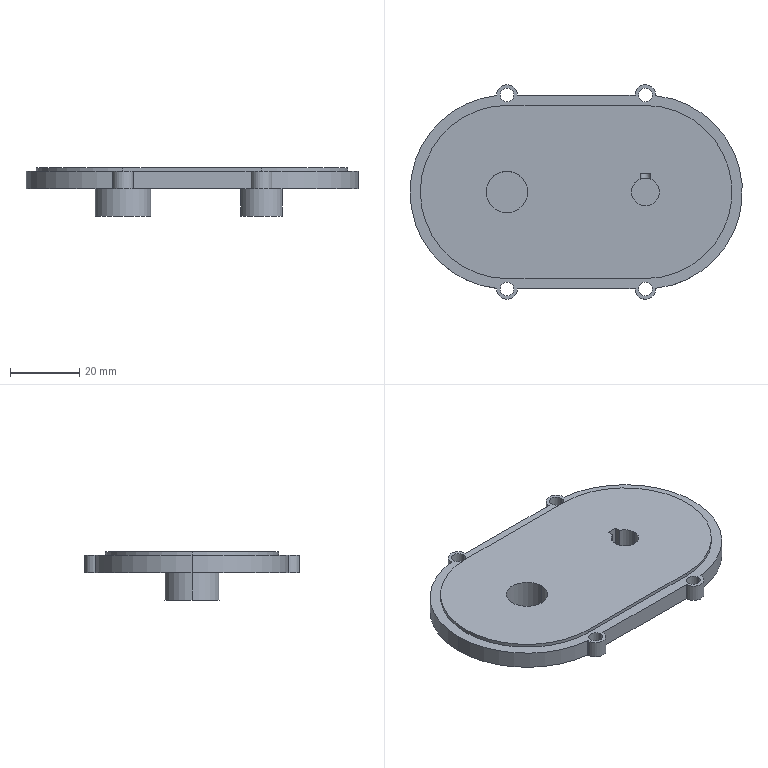Part | SolidWorks | features ICE 6, Extrusion 1 | 1 solid | 43 faces | box 96 x 62 x 14 mm | volume 28190 mm3 | cylinder 29 | plane 14 | commonest cylinder face diameters 4 x8 6 x6 12 x4 50 x3 56 x3 8 x2
STEP:
#1=CARTESIAN_POINT('',(-26.,0.,-5.));
#2=VERTEX_POINT('',#1);
#3=CARTESIAN_POINT('',(-14.,0.,-5.));
#4=VERTEX_POINT('',#3);
#5=CARTESIAN_POINT('',(-20.,0.,-5.));
#6=DIRECTION('',(0.,0.,1.));
#7=DIRECTION('',(1.,0.,0.));
#8=AXIS2_PLACEMENT_3D('',#5,#6,#7);
#9=CIRCLE('',#8,6.);
#10=EDGE_CURVE('',#2,#4,#9,.T.);
#11=ORIENTED_EDGE('',*,*,#10,.F.);
#12=CARTESIAN_POINT('',(-26.,0.,6.));
#13=VERTEX_POINT('',#12);
#14=CARTESIAN_POINT('',(-26.,0.,-5.));
#15=DIRECTION('',(0.,0.,1.));
#16=VECTOR('',#15,1000.);
#17=LINE('',#14,#16);
#18=EDGE_CURVE('',#2,#13,#17,.T.);
#19=ORIENTED_EDGE('',*,*,#18,.T.);
#20=CARTESIAN_POINT('',(-14.,0.,6.));
#21=VERTEX_POINT('',#20);
#22=CARTESIAN_POINT('',(-20.,0.,6.));
#23=DIRECTION('',(0.,0.,1.));
#24=DIRECTION('',(1.,0.,0.));
#25=AXIS2_PLACEMENT_3D('',#22,#23,#24);
#26=CIRCLE('',#25,6.);
#27=EDGE_CURVE('',#13,#21,#26,.T.);
#28=ORIENTED_EDGE('',*,*,#27,.T.);
#29=CARTESIAN_POINT('',(-14.,0.,-5.));
#30=DIRECTION('',(0.,0.,1.));
#31=VECTOR('',#30,1000.);
#32=LINE('',#29,#31);
#33=EDGE_CURVE('',#4,#21,#32,.T.);
#34=ORIENTED_EDGE('',*,*,#33,.F.);
#35=EDGE_LOOP('',(#11,#19,#28,#34));
#36=FACE_OUTER_BOUND('',#35,.T.);
#37=CARTESIAN_POINT('',(-20.,0.,-5.));
#38=DIRECTION('',(0.,0.,1.));
#39=DIRECTION('',(1.,0.,0.));
#40=AXIS2_PLACEMENT_3D('',#37,#38,#39);
#41=CYLINDRICAL_SURFACE('',#40,6.);
#42=ADVANCED_FACE('',(#36),#41,.F.);
#43=CARTESIAN_POINT('',(16.,0.,-5.));
#44=VERTEX_POINT('',#43);
#45=CARTESIAN_POINT('',(24.,0.,-5.));
#46=VERTEX_POINT('',#45);
#47=CARTESIAN_POINT('',(20.,0.,-5.));
#48=DIRECTION('',(0.,0.,1.));
#49=DIRECTION('',(1.,0.,0.));
#50=AXIS2_PLACEMENT_3D('',#47,#48,#49);
#51=CIRCLE('',#50,4.);
#52=EDGE_CURVE('',#44,#46,#51,.T.);
#53=ORIENTED_EDGE('',*,*,#52,.F.);
#54=CARTESIAN_POINT('',(16.,0.,6.));
#55=VERTEX_POINT('',#54);
#56=CARTESIAN_POINT('',(16.,0.,-5.));
#57=DIRECTION('',(0.,0.,1.));
#58=VECTOR('',#57,1000.);
#59=LINE('',#56,#58);
#60=EDGE_CURVE('',#44,#55,#59,.T.);
#61=ORIENTED_EDGE('',*,*,#60,.T.);
#62=CARTESIAN_POINT('',(24.,0.,6.));
#63=VERTEX_POINT('',#62);
#64=CARTESIAN_POINT('',(20.,0.,6.));
#65=DIRECTION('',(0.,0.,1.));
#66=DIRECTION('',(1.,0.,0.));
#67=AXIS2_PLACEMENT_3D('',#64,#65,#66);
#68=CIRCLE('',#67,4.);
#69=EDGE_CURVE('',#55,#63,#68,.T.);
#70=ORIENTED_EDGE('',*,*,#69,.T.);
#71=CARTESIAN_POINT('',(24.,0.,-5.));
#72=DIRECTION('',(0.,0.,1.));
#73=VECTOR('',#72,1000.);
#74=LINE('',#71,#73);
#75=EDGE_CURVE('',#46,#63,#74,.T.);
#76=ORIENTED_EDGE('',*,*,#75,.F.);
#77=EDGE_LOOP('',(#53,#61,#70,#76));
#78=FACE_OUTER_BOUND('',#77,.T.);
#79=CARTESIAN_POINT('',(20.,0.,-5.));
#80=DIRECTION('',(0.,0.,1.));
#81=DIRECTION('',(1.,0.,0.));
#82=AXIS2_PLACEMENT_3D('',#79,#80,#81);
#83=CYLINDRICAL_SURFACE('',#82,4.);
#84=ADVANCED_FACE('',(#78),#83,.F.);
#85=CARTESIAN_POINT('',(-28.,0.,-8.));
#86=VERTEX_POINT('',#85);
#87=CARTESIAN_POINT('',(-12.,0.,-8.));
#88=VERTEX_POINT('',#87);
#89=CARTESIAN_POINT('',(-20.,0.,-8.));
#90=DIRECTION('',(0.,0.,-1.));
#91=DIRECTION('',(-1.,0.,0.));
#92=AXIS2_PLACEMENT_3D('',#89,#90,#91);
#93=CIRCLE('',#92,8.);
#94=EDGE_CURVE('',#86,#88,#93,.T.);
#95=ORIENTED_EDGE('',*,*,#94,.F.);
#96=CARTESIAN_POINT('',(-28.,0.,0.));
#97=VERTEX_POINT('',#96);
#98=CARTESIAN_POINT('',(-28.,0.,-8.));
#99=DIRECTION('',(0.,0.,1.));
#100=VECTOR('',#99,1000.);
#101=LINE('',#98,#100);
#102=EDGE_CURVE('',#86,#97,#101,.T.);
#103=ORIENTED_EDGE('',*,*,#102,.T.);
#104=CARTESIAN_POINT('',(-12.,0.,0.));
#105=VERTEX_POINT('',#104);
#106=CARTESIAN_POINT('',(-20.,0.,0.));
#107=DIRECTION('',(0.,0.,-1.));
#108=DIRECTION('',(1.,0.,0.));
#109=AXIS2_PLACEMENT_3D('',#106,#107,#108);
#110=CIRCLE('',#109,8.);
#111=EDGE_CURVE('',#97,#105,#110,.T.);
#112=ORIENTED_EDGE('',*,*,#111,.T.);
#113=CARTESIAN_POINT('',(-12.,0.,-8.));
#114=DIRECTION('',(0.,0.,1.));
#115=VECTOR('',#114,1000.);
#116=LINE('',#113,#115);
#117=EDGE_CURVE('',#88,#105,#116,.T.);
#118=ORIENTED_EDGE('',*,*,#117,.F.);
#119=EDGE_LOOP('',(#95,#103,#112,#118));
#120=FACE_OUTER_BOUND('',#119,.T.);
#121=CARTESIAN_POINT('',(-20.,0.,-8.));
#122=DIRECTION('',(0.,0.,1.));
#123=DIRECTION('',(1.,0.,0.));
#124=AXIS2_PLACEMENT_3D('',#121,#122,#123);
#125=CYLINDRICAL_SURFACE('',#124,8.);
#126=ADVANCED_FACE('',(#120),#125,.T.);
#127=CARTESIAN_POINT('',(14.,0.,-8.));
#128=VERTEX_POINT('',#127);
#129=CARTESIAN_POINT('',(26.,0.,-8.));
#130=VERTEX_POINT('',#129);
#131=CARTESIAN_POINT('',(20.,0.,-8.));
#132=DIRECTION('',(0.,0.,-1.));
#133=DIRECTION('',(-1.,0.,0.));
#134=AXIS2_PLACEMENT_3D('',#131,#132,#133);
#135=CIRCLE('',#134,6.);
#136=EDGE_CURVE('',#128,#130,#135,.T.);
#137=ORIENTED_EDGE('',*,*,#136,.F.);
#138=CARTESIAN_POINT('',(14.,0.,0.));
#139=VERTEX_POINT('',#138);
#140=CARTESIAN_POINT('',(14.,0.,-8.));
#141=DIRECTION('',(0.,0.,1.));
#142=VECTOR('',#141,1000.);
#143=LINE('',#140,#142);
#144=EDGE_CURVE('',#128,#139,#143,.T.);
#145=ORIENTED_EDGE('',*,*,#144,.T.);
#146=CARTESIAN_POINT('',(26.,0.,0.));
#147=VERTEX_POINT('',#146);
#148=CARTESIAN_POINT('',(20.,0.,0.));
#149=DIRECTION('',(0.,0.,-1.));
#150=DIRECTION('',(1.,0.,0.));
#151=AXIS2_PLACEMENT_3D('',#148,#149,#150);
#152=CIRCLE('',#151,6.);
#153=EDGE_CURVE('',#139,#147,#152,.T.);
#154=ORIENTED_EDGE('',*,*,#153,.T.);
#155=CARTESIAN_POINT('',(26.,0.,-8.));
#156=DIRECTION('',(0.,0.,1.));
#157=VECTOR('',#156,1000.);
#158=LINE('',#155,#157);
#159=EDGE_CURVE('',#130,#147,#158,.T.);
#160=ORIENTED_EDGE('',*,*,#159,.F.);
#161=EDGE_LOOP('',(#137,#145,#154,#160));
#162=FACE_OUTER_BOUND('',#161,.T.);
#163=CARTESIAN_POINT('',(20.,0.,-8.));
#164=DIRECTION('',(0.,0.,1.));
#165=DIRECTION('',(1.,0.,0.));
#166=AXIS2_PLACEMENT_3D('',#163,#164,#165);
#167=CYLINDRICAL_SURFACE('',#166,6.);
#168=ADVANCED_FACE('',(#162),#167,.T.);
#169=CARTESIAN_POINT('',(-18.,28.,5.));
#170=VERTEX_POINT('',#169);
#171=CARTESIAN_POINT('',(-22.,28.,5.));
#172=VERTEX_POINT('',#171);
#173=CARTESIAN_POINT('',(-20.,28.,5.));
#174=DIRECTION('',(0.,0.,-1.));
#175=DIRECTION('',(-1.,0.,0.));
#176=AXIS2_PLACEMENT_3D('',#173,#174,#175);
#177=CIRCLE('',#176,2.);
#178=EDGE_CURVE('',#170,#172,#177,.T.);
#179=ORIENTED_EDGE('',*,*,#178,.F.);
#180=CARTESIAN_POINT('',(-18.,28.,0.));
#181=VERTEX_POINT('',#180);
#182=CARTESIAN_POINT('',(-18.,28.,5.));
#183=DIRECTION('',(0.,0.,-1.));
#184=VECTOR('',#183,1000.);
#185=LINE('',#182,#184);
#186=EDGE_CURVE('',#170,#181,#185,.T.);
#187=ORIENTED_EDGE('',*,*,#186,.T.);
#188=CARTESIAN_POINT('',(-22.,28.,0.));
#189=VERTEX_POINT('',#188);
#190=CARTESIAN_POINT('',(-20.,28.,0.));
#191=DIRECTION('',(0.,0.,-1.));
#192=DIRECTION('',(-1.,0.,0.));
#193=AXIS2_PLACEMENT_3D('',#190,#191,#192);
#194=CIRCLE('',#193,2.);
#195=EDGE_CURVE('',#181,#189,#194,.T.);
#196=ORIENTED_EDGE('',*,*,#195,.T.);
#197=CARTESIAN_POINT('',(-22.,28.,5.));
#198=DIRECTION('',(0.,0.,-1.));
#199=VECTOR('',#198,1000.);
#200=LINE('',#197,#199);
#201=EDGE_CURVE('',#172,#189,#200,.T.);
#202=ORIENTED_EDGE('',*,*,#201,.F.);
#203=EDGE_LOOP('',(#179,#187,#196,#202));
#204=FACE_OUTER_BOUND('',#203,.T.);
#205=CARTESIAN_POINT('',(-20.,28.,5.));
#206=DIRECTION('',(0.,0.,-1.));
#207=DIRECTION('',(-1.,0.,0.));
#208=AXIS2_PLACEMENT_3D('',#205,#206,#207);
#209=CYLINDRICAL_SURFACE('',#208,2.);
#210=ADVANCED_FACE('',(#204),#209,.F.);
#211=CARTESIAN_POINT('',(22.,-28.,5.));
#212=VERTEX_POINT('',#211);
#213=CARTESIAN_POINT('',(18.,-28.,5.));
#214=VERTEX_POINT('',#213);
#215=CARTESIAN_POINT('',(20.,-28.,5.));
#216=DIRECTION('',(0.,0.,-1.));
#217=DIRECTION('',(-1.,0.,0.));
#218=AXIS2_PLACEMENT_3D('',#215,#216,#217);
#219=CIRCLE('',#218,2.);
#220=EDGE_CURVE('',#212,#214,#219,.T.);
#221=ORIENTED_EDGE('',*,*,#220,.F.);
#222=CARTESIAN_POINT('',(22.,-28.,0.));
#223=VERTEX_POINT('',#222);
#224=CARTESIAN_POINT('',(22.,-28.,5.));
#225=DIRECTION('',(0.,0.,-1.));
#226=VECTOR('',#225,1000.);
#227=LINE('',#224,#226);
#228=EDGE_CURVE('',#212,#223,#227,.T.);
#229=ORIENTED_EDGE('',*,*,#228,.T.);
#230=CARTESIAN_POINT('',(18.,-28.,0.));
#231=VERTEX_POINT('',#230);
#232=CARTESIAN_POINT('',(20.,-28.,0.));
#233=DIRECTION('',(0.,0.,-1.));
#234=DIRECTION('',(-1.,0.,0.));
#235=AXIS2_PLACEMENT_3D('',#232,#233,#234);
#236=CIRCLE('',#235,2.);
#237=EDGE_CURVE('',#223,#231,#236,.T.);
#238=ORIENTED_EDGE('',*,*,#237,.T.);
#239=CARTESIAN_POINT('',(18.,-28.,5.));
#240=DIRECTION('',(0.,0.,-1.));
#241=VECTOR('',#240,1000.);
#242=LINE('',#239,#241);
#243=EDGE_CURVE('',#214,#231,#242,.T.);
#244=ORIENTED_EDGE('',*,*,#243,.F.);
#245=EDGE_LOOP('',(#221,#229,#238,#244));
#246=FACE_OUTER_BOUND('',#245,.T.);
#247=CARTESIAN_POINT('',(20.,-28.,5.));
#248=DIRECTION('',(0.,0.,-1.));
#249=DIRECTION('',(-1.,0.,0.));
#250=AXIS2_PLACEMENT_3D('',#247,#248,#249);
#251=CYLINDRICAL_SURFACE('',#250,2.);
#252=ADVANCED_FACE('',(#246),#251,.F.);
#253=CARTESIAN_POINT('',(-18.,-28.,5.));
#254=VERTEX_POINT('',#253);
#255=CARTESIAN_POINT('',(-22.,-28.,5.));
#256=VERTEX_POINT('',#255);
#257=CARTESIAN_POINT('',(-20.,-28.,5.));
#258=DIRECTION('',(0.,0.,-1.));
#259=DIRECTION('',(-1.,0.,0.));
#260=AXIS2_PLACEMENT_3D('',#257,#258,#259);
#261=CIRCLE('',#260,2.);
#262=EDGE_CURVE('',#254,#256,#261,.T.);
#263=ORIENTED_EDGE('',*,*,#262,.F.);
#264=CARTESIAN_POINT('',(-18.,-28.,0.));
#265=VERTEX_POINT('',#264);
#266=CARTESIAN_POINT('',(-18.,-28.,5.));
#267=DIRECTION('',(0.,0.,-1.));
#268=VECTOR('',#267,1000.);
#269=LINE('',#266,#268);
#270=EDGE_CURVE('',#254,#265,#269,.T.);
#271=ORIENTED_EDGE('',*,*,#270,.T.);
#272=CARTESIAN_POINT('',(-22.,-28.,0.));
#273=VERTEX_POINT('',#272);
#274=CARTESIAN_POINT('',(-20.,-28.,0.));
#275=DIRECTION('',(0.,0.,-1.));
#276=DIRECTION('',(-1.,0.,0.));
#277=AXIS2_PLACEMENT_3D('',#274,#275,#276);
#278=CIRCLE('',#277,2.);
#279=EDGE_CURVE('',#265,#273,#278,.T.);
#280=ORIENTED_EDGE('',*,*,#279,.T.);
#281=CARTESIAN_POINT('',(-22.,-28.,5.));
#282=DIRECTION('',(0.,0.,-1.));
#283=VECTOR('',#282,1000.);
#284=LINE('',#281,#283);
#285=EDGE_CURVE('',#256,#273,#284,.T.);
#286=ORIENTED_EDGE('',*,*,#285,.F.);
#287=EDGE_LOOP('',(#263,#271,#280,#286));
#288=FACE_OUTER_BOUND('',#287,.T.);
#289=CARTESIAN_POINT('',(-20.,-28.,5.));
#290=DIRECTION('',(0.,0.,-1.));
#291=DIRECTION('',(-1.,0.,0.));
#292=AXIS2_PLACEMENT_3D('',#289,#290,#291);
#293=CYLINDRICAL_SURFACE('',#292,2.);
#294=ADVANCED_FACE('',(#288),#293,.F.);
#295=CARTESIAN_POINT('',(22.,28.,5.));
#296=VERTEX_POINT('',#295);
#297=CARTESIAN_POINT('',(18.,28.,5.));
#298=VERTEX_POINT('',#297);
#299=CARTESIAN_POINT('',(20.,28.,5.));
#300=DIRECTION('',(0.,0.,-1.));
#301=DIRECTION('',(-1.,0.,0.));
#302=AXIS2_PLACEMENT_3D('',#299,#300,#301);
#303=CIRCLE('',#302,2.);
#304=EDGE_CURVE('',#296,#298,#303,.T.);
#305=ORIENTED_EDGE('',*,*,#304,.F.);
#306=CARTESIAN_POINT('',(22.,28.,0.));
#307=VERTEX_POINT('',#306);
#308=CARTESIAN_POINT('',(22.,28.,5.));
#309=DIRECTION('',(0.,0.,-1.));
#310=VECTOR('',#309,1000.);
#311=LINE('',#308,#310);
#312=EDGE_CURVE('',#296,#307,#311,.T.);
#313=ORIENTED_EDGE('',*,*,#312,.T.);
#314=CARTESIAN_POINT('',(18.,28.,0.));
#315=VERTEX_POINT('',#314);
#316=CARTESIAN_POINT('',(20.,28.,0.));
#317=DIRECTION('',(0.,0.,-1.));
#318=DIRECTION('',(-1.,0.,0.));
#319=AXIS2_PLACEMENT_3D('',#316,#317,#318);
#320=CIRCLE('',#319,2.);
#321=EDGE_CURVE('',#307,#315,#320,.T.);
#322=ORIENTED_EDGE('',*,*,#321,.T.);
#323=CARTESIAN_POINT('',(18.,28.,5.));
#324=DIRECTION('',(0.,0.,-1.));
#325=VECTOR('',#324,1000.);
#326=LINE('',#323,#325);
#327=EDGE_CURVE('',#298,#315,#326,.T.);
#328=ORIENTED_EDGE('',*,*,#327,.F.);
#329=EDGE_LOOP('',(#305,#313,#322,#328));
#330=FACE_OUTER_BOUND('',#329,.T.);
#331=CARTESIAN_POINT('',(20.,28.,5.));
#332=DIRECTION('',(0.,0.,-1.));
#333=DIRECTION('',(-1.,0.,0.));
#334=AXIS2_PLACEMENT_3D('',#331,#332,#333);
#335=CYLINDRICAL_SURFACE('',#334,2.);
#336=ADVANCED_FACE('',(#330),#335,.F.);
#337=CARTESIAN_POINT('',(-17.,-28.,5.));
#338=VERTEX_POINT('',#337);
#339=CARTESIAN_POINT('',(-23.,-28.,5.));
#340=VERTEX_POINT('',#339);
#341=CARTESIAN_POINT('',(-20.,-28.,5.));
#342=DIRECTION('',(0.,0.,-1.));
#343=DIRECTION('',(-1.,0.,0.));
#344=AXIS2_PLACEMENT_3D('',#341,#342,#343);
#345=CIRCLE('',#344,3.);
#346=EDGE_CURVE('',#338,#340,#345,.T.);
#347=ORIENTED_EDGE('',*,*,#346,.T.);
#348=CARTESIAN_POINT('',(-23.,-28.,0.));
#349=VERTEX_POINT('',#348);
#350=CARTESIAN_POINT('',(-23.,-28.,5.));
#351=DIRECTION('',(0.,0.,-1.));
#352=VECTOR('',#351,1000.);
#353=LINE('',#350,#352);
#354=EDGE_CURVE('',#340,#349,#353,.T.);
#355=ORIENTED_EDGE('',*,*,#354,.T.);
#356=CARTESIAN_POINT('',(-17.,-28.,0.));
#357=VERTEX_POINT('',#356);
#358=CARTESIAN_POINT('',(-20.,-28.,0.));
#359=DIRECTION('',(0.,0.,-1.));
#360=DIRECTION('',(-1.,0.,0.));
#361=AXIS2_PLACEMENT_3D('',#358,#359,#360);
#362=CIRCLE('',#361,3.);
#363=EDGE_CURVE('',#357,#349,#362,.T.);
#364=ORIENTED_EDGE('',*,*,#363,.F.);
#365=CARTESIAN_POINT('',(-17.,-28.,5.));
#366=DIRECTION('',(0.,0.,-1.));
#367=VECTOR('',#366,1000.);
#368=LINE('',#365,#367);
#369=EDGE_CURVE('',#338,#357,#368,.T.);
#370=ORIENTED_EDGE('',*,*,#369,.F.);
#371=EDGE_LOOP('',(#347,#355,#364,#370));
#372=FACE_OUTER_BOUND('',#371,.T.);
#373=CARTESIAN_POINT('',(-20.,-28.,5.));
#374=DIRECTION('',(0.,0.,-1.));
#375=DIRECTION('',(-1.,0.,0.));
#376=AXIS2_PLACEMENT_3D('',#373,#374,#375);
#377=CYLINDRICAL_SURFACE('',#376,3.);
#378=ADVANCED_FACE('',(#372),#377,.T.);
#379=CARTESIAN_POINT('',(-22.996,27.839,5.));
#380=VERTEX_POINT('',#379);
#381=CARTESIAN_POINT('',(-23.,28.,5.));
#382=VERTEX_POINT('',#381);
#383=CARTESIAN_POINT('',(-20.,28.,5.));
#384=DIRECTION('',(0.,0.,-1.));
#385=DIRECTION('',(-1.,0.,0.));
#386=AXIS2_PLACEMENT_3D('',#383,#384,#385);
#387=CIRCLE('',#386,3.);
#388=EDGE_CURVE('',#380,#382,#387,.T.);
#389=ORIENTED_EDGE('',*,*,#388,.T.);
#390=CARTESIAN_POINT('',(-23.,28.,0.));
#391=VERTEX_POINT('',#390);
#392=CARTESIAN_POINT('',(-23.,28.,5.));
#393=DIRECTION('',(0.,0.,-1.));
#394=VECTOR('',#393,1000.);
#395=LINE('',#392,#394);
#396=EDGE_CURVE('',#382,#391,#395,.T.);
#397=ORIENTED_EDGE('',*,*,#396,.T.);
#398=CARTESIAN_POINT('',(-22.996,27.839,0.));
#399=VERTEX_POINT('',#398);
#400=CARTESIAN_POINT('',(-20.,28.,0.));
#401=DIRECTION('',(0.,0.,-1.));
#402=DIRECTION('',(-1.,0.,0.));
#403=AXIS2_PLACEMENT_3D('',#400,#401,#402);
#404=CIRCLE('',#403,3.);
#405=EDGE_CURVE('',#399,#391,#404,.T.);
#406=ORIENTED_EDGE('',*,*,#405,.F.);
#407=CARTESIAN_POINT('',(-22.996,27.839,2.5));
#408=DIRECTION('',(0.,0.,-1.));
#409=VECTOR('',#408,1000.);
#410=LINE('',#407,#409);
#411=EDGE_CURVE('',#380,#399,#410,.T.);
#412=ORIENTED_EDGE('',*,*,#411,.F.);
#413=EDGE_LOOP('',(#389,#397,#406,#412));
#414=FACE_OUTER_BOUND('',#413,.T.);
#415=CARTESIAN_POINT('',(-20.,28.,5.));
#416=DIRECTION('',(0.,0.,-1.));
#417=DIRECTION('',(-1.,0.,0.));
#418=AXIS2_PLACEMENT_3D('',#415,#416,#417);
#419=CYLINDRICAL_SURFACE('',#418,3.);
#420=ADVANCED_FACE('',(#414),#419,.T.);
#421=CARTESIAN_POINT('',(-45.,0.,6.));
#422=VERTEX_POINT('',#421);
#423=CARTESIAN_POINT('',(-20.,-25.,6.));
#424=VERTEX_POINT('',#423);
#425=CARTESIAN_POINT('',(-20.,0.,6.));
#426=DIRECTION('',(0.,0.,1.));
#427=DIRECTION('',(1.,0.,0.));
#428=AXIS2_PLACEMENT_3D('',#425,#426,#427);
#429=CIRCLE('',#428,25.);
#430=EDGE_CURVE('',#422,#424,#429,.T.);
#431=ORIENTED_EDGE('',*,*,#430,.F.);
#432=CARTESIAN_POINT('',(-45.,0.,5.));
#433=VERTEX_POINT('',#432);
#434=CARTESIAN_POINT('',(-45.,0.,6.));
#435=DIRECTION('',(0.,0.,-1.));
#436=VECTOR('',#435,1000.);
#437=LINE('',#434,#436);
#438=EDGE_CURVE('',#422,#433,#437,.T.);
#439=ORIENTED_EDGE('',*,*,#438,.T.);
#440=CARTESIAN_POINT('',(-20.,-25.,5.));
#441=VERTEX_POINT('',#440);
#442=CARTESIAN_POINT('',(-20.,0.,5.));
#443=DIRECTION('',(0.,0.,1.));
#444=DIRECTION('',(1.,0.,0.));
#445=AXIS2_PLACEMENT_3D('',#442,#443,#444);
#446=CIRCLE('',#445,25.);
#447=EDGE_CURVE('',#433,#441,#446,.T.);
#448=ORIENTED_EDGE('',*,*,#447,.T.);
#449=CARTESIAN_POINT('',(-20.,-25.,6.));
#450=DIRECTION('',(0.,0.,-1.));
#451=VECTOR('',#450,1000.);
#452=LINE('',#449,#451);
#453=EDGE_CURVE('',#424,#441,#452,.T.);
#454=ORIENTED_EDGE('',*,*,#453,.F.);
#455=EDGE_LOOP('',(#431,#439,#448,#454));
#456=FACE_OUTER_BOUND('',#455,.T.);
#457=CARTESIAN_POINT('',(-20.,0.,6.));
#458=DIRECTION('',(0.,0.,-1.));
#459=DIRECTION('',(-1.,0.,0.));
#460=AXIS2_PLACEMENT_3D('',#457,#458,#459);
#461=CYLINDRICAL_SURFACE('',#460,25.);
#462=ADVANCED_FACE('',(#456),#461,.T.);
#463=CARTESIAN_POINT('',(-48.,0.,5.));
#464=VERTEX_POINT('',#463);
#465=CARTESIAN_POINT('',(-22.996,-27.839,5.));
#466=VERTEX_POINT('',#465);
#467=CARTESIAN_POINT('',(-20.,0.,5.));
#468=DIRECTION('',(0.,0.,1.));
#469=DIRECTION('',(1.,0.,0.));
#470=AXIS2_PLACEMENT_3D('',#467,#468,#469);
#471=CIRCLE('',#470,28.);
#472=EDGE_CURVE('',#464,#466,#471,.T.);
#473=ORIENTED_EDGE('',*,*,#472,.F.);
#474=CARTESIAN_POINT('',(-48.,0.,0.));
#475=VERTEX_POINT('',#474);
#476=CARTESIAN_POINT('',(-48.,0.,5.));
#477=DIRECTION('',(0.,0.,-1.));
#478=VECTOR('',#477,1000.);
#479=LINE('',#476,#478);
#480=EDGE_CURVE('',#464,#475,#479,.T.);
#481=ORIENTED_EDGE('',*,*,#480,.T.);
#482=CARTESIAN_POINT('',(-22.996,-27.839,0.));
#483=VERTEX_POINT('',#482);
#484=CARTESIAN_POINT('',(-20.,0.,0.));
#485=DIRECTION('',(0.,0.,1.));
#486=DIRECTION('',(1.,0.,0.));
#487=AXIS2_PLACEMENT_3D('',#484,#485,#486);
#488=CIRCLE('',#487,28.);
#489=EDGE_CURVE('',#475,#483,#488,.T.);
#490=ORIENTED_EDGE('',*,*,#489,.T.);
#491=CARTESIAN_POINT('',(-22.996,-27.839,2.5));
#492=DIRECTION('',(0.,0.,1.));
#493=VECTOR('',#492,1000.);
#494=LINE('',#491,#493);
#495=EDGE_CURVE('',#483,#466,#494,.T.);
#496=ORIENTED_EDGE('',*,*,#495,.T.);
#497=EDGE_LOOP('',(#473,#481,#490,#496));
#498=FACE_OUTER_BOUND('',#497,.T.);
#499=CARTESIAN_POINT('',(-20.,0.,5.));
#500=DIRECTION('',(0.,0.,-1.));
#501=DIRECTION('',(-1.,0.,0.));
#502=AXIS2_PLACEMENT_3D('',#499,#500,#501);
#503=CYLINDRICAL_SURFACE('',#502,28.);
#504=ADVANCED_FACE('',(#498),#503,.T.);
#505=ORIENTED_EDGE('',*,*,#480,.F.);
#506=CARTESIAN_POINT('',(-20.,0.,5.));
#507=DIRECTION('',(0.,0.,1.));
#508=DIRECTION('',(1.,0.,0.));
#509=AXIS2_PLACEMENT_3D('',#506,#507,#508);
#510=CIRCLE('',#509,28.);
#511=EDGE_CURVE('',#380,#464,#510,.T.);
#512=ORIENTED_EDGE('',*,*,#511,.F.);
#513=ORIENTED_EDGE('',*,*,#411,.T.);
#514=CARTESIAN_POINT('',(-20.,0.,0.));
#515=DIRECTION('',(0.,0.,1.));
#516=DIRECTION('',(1.,0.,0.));
#517=AXIS2_PLACEMENT_3D('',#514,#515,#516);
#518=CIRCLE('',#517,28.);
#519=EDGE_CURVE('',#399,#475,#518,.T.);
#520=ORIENTED_EDGE('',*,*,#519,.T.);
#521=EDGE_LOOP('',(#505,#512,#513,#520));
#522=FACE_OUTER_BOUND('',#521,.T.);
#523=CARTESIAN_POINT('',(-20.,0.,5.));
#524=DIRECTION('',(0.,0.,-1.));
#525=DIRECTION('',(-1.,0.,0.));
#526=AXIS2_PLACEMENT_3D('',#523,#524,#525);
#527=CYLINDRICAL_SURFACE('',#526,28.);
#528=ADVANCED_FACE('',(#522),#527,.T.);
#529=CARTESIAN_POINT('',(17.,-28.,5.));
#530=VERTEX_POINT('',#529);
#531=CARTESIAN_POINT('',(-20.,-28.,5.));
#532=DIRECTION('',(1.,0.,0.));
#533=VECTOR('',#532,1000.);
#534=LINE('',#531,#533);
#535=EDGE_CURVE('',#338,#530,#534,.T.);
#536=ORIENTED_EDGE('',*,*,#535,.F.);
#537=ORIENTED_EDGE('',*,*,#369,.T.);
#538=CARTESIAN_POINT('',(17.,-28.,0.));
#539=VERTEX_POINT('',#538);
#540=CARTESIAN_POINT('',(-20.,-28.,0.));
#541=DIRECTION('',(1.,0.,0.));
#542=VECTOR('',#541,1000.);
#543=LINE('',#540,#542);
#544=EDGE_CURVE('',#357,#539,#543,.T.);
#545=ORIENTED_EDGE('',*,*,#544,.T.);
#546=CARTESIAN_POINT('',(17.,-28.,5.));
#547=DIRECTION('',(0.,0.,1.));
#548=VECTOR('',#547,1000.);
#549=LINE('',#546,#548);
#550=EDGE_CURVE('',#539,#530,#549,.T.);
#551=ORIENTED_EDGE('',*,*,#550,.T.);
#552=EDGE_LOOP('',(#536,#537,#545,#551));
#553=FACE_OUTER_BOUND('',#552,.T.);
#554=CARTESIAN_POINT('',(-20.,-28.,5.));
#555=DIRECTION('',(0.,1.,0.));
#556=DIRECTION('',(0.,0.,1.));
#557=AXIS2_PLACEMENT_3D('',#554,#555,#556);
#558=PLANE('',#557);
#559=ADVANCED_FACE('',(#553),#558,.F.);
#560=CARTESIAN_POINT('',(22.996,-27.839,5.));
#561=VERTEX_POINT('',#560);
#562=CARTESIAN_POINT('',(22.996,27.839,5.));
#563=VERTEX_POINT('',#562);
#564=CARTESIAN_POINT('',(20.,0.,5.));
#565=DIRECTION('',(0.,0.,1.));
#566=DIRECTION('',(1.,0.,0.));
#567=AXIS2_PLACEMENT_3D('',#564,#565,#566);
#568=CIRCLE('',#567,28.);
#569=EDGE_CURVE('',#561,#563,#568,.T.);
#570=ORIENTED_EDGE('',*,*,#569,.F.);
#571=CARTESIAN_POINT('',(22.996,-27.839,0.));
#572=VERTEX_POINT('',#571);
#573=CARTESIAN_POINT('',(22.996,-27.839,2.5));
#574=DIRECTION('',(0.,0.,-1.));
#575=VECTOR('',#574,1000.);
#576=LINE('',#573,#575);
#577=EDGE_CURVE('',#561,#572,#576,.T.);
#578=ORIENTED_EDGE('',*,*,#577,.T.);
#579=CARTESIAN_POINT('',(22.996,27.839,0.));
#580=VERTEX_POINT('',#579);
#581=CARTESIAN_POINT('',(20.,0.,0.));
#582=DIRECTION('',(0.,0.,1.));
#583=DIRECTION('',(1.,0.,0.));
#584=AXIS2_PLACEMENT_3D('',#581,#582,#583);
#585=CIRCLE('',#584,28.);
#586=EDGE_CURVE('',#572,#580,#585,.T.);
#587=ORIENTED_EDGE('',*,*,#586,.T.);
#588=CARTESIAN_POINT('',(22.996,27.839,2.5));
#589=DIRECTION('',(0.,0.,1.));
#590=VECTOR('',#589,1000.);
#591=LINE('',#588,#590);
#592=EDGE_CURVE('',#580,#563,#591,.T.);
#593=ORIENTED_EDGE('',*,*,#592,.T.);
#594=EDGE_LOOP('',(#570,#578,#587,#593));
#595=FACE_OUTER_BOUND('',#594,.T.);
#596=CARTESIAN_POINT('',(20.,0.,5.));
#597=DIRECTION('',(0.,0.,-1.));
#598=DIRECTION('',(-1.,0.,0.));
#599=AXIS2_PLACEMENT_3D('',#596,#597,#598);
#600=CYLINDRICAL_SURFACE('',#599,28.);
#601=ADVANCED_FACE('',(#595),#600,.T.);
#602=CARTESIAN_POINT('',(17.,28.,0.));
#603=VERTEX_POINT('',#602);
#604=CARTESIAN_POINT('',(-17.,28.,0.));
#605=VERTEX_POINT('',#604);
#606=CARTESIAN_POINT('',(-20.,28.,0.));
#607=DIRECTION('',(-1.,0.,0.));
#608=VECTOR('',#607,1000.);
#609=LINE('',#606,#608);
#610=EDGE_CURVE('',#603,#605,#609,.T.);
#611=ORIENTED_EDGE('',*,*,#610,.T.);
#612=CARTESIAN_POINT('',(-17.,28.,5.));
#613=VERTEX_POINT('',#612);
#614=CARTESIAN_POINT('',(-17.,28.,5.));
#615=DIRECTION('',(0.,0.,1.));
#616=VECTOR('',#615,1000.);
#617=LINE('',#614,#616);
#618=EDGE_CURVE('',#605,#613,#617,.T.);
#619=ORIENTED_EDGE('',*,*,#618,.T.);
#620=CARTESIAN_POINT('',(17.,28.,5.));
#621=VERTEX_POINT('',#620);
#622=CARTESIAN_POINT('',(-20.,28.,5.));
#623=DIRECTION('',(-1.,0.,0.));
#624=VECTOR('',#623,1000.);
#625=LINE('',#622,#624);
#626=EDGE_CURVE('',#621,#613,#625,.T.);
#627=ORIENTED_EDGE('',*,*,#626,.F.);
#628=CARTESIAN_POINT('',(17.,28.,5.));
#629=DIRECTION('',(0.,0.,-1.));
#630=VECTOR('',#629,1000.);
#631=LINE('',#628,#630);
#632=EDGE_CURVE('',#621,#603,#631,.T.);
#633=ORIENTED_EDGE('',*,*,#632,.T.);
#634=EDGE_LOOP('',(#611,#619,#627,#633));
#635=FACE_OUTER_BOUND('',#634,.T.);
#636=CARTESIAN_POINT('',(-20.,28.,5.));
#637=DIRECTION('',(0.,-1.,0.));
#638=DIRECTION('',(0.,0.,-1.));
#639=AXIS2_PLACEMENT_3D('',#636,#637,#638);
#640=PLANE('',#639);
#641=ADVANCED_FACE('',(#635),#640,.F.);
#642=CARTESIAN_POINT('',(-20.,28.,5.));
#643=DIRECTION('',(0.,0.,-1.));
#644=DIRECTION('',(-1.,0.,0.));
#645=AXIS2_PLACEMENT_3D('',#642,#643,#644);
#646=CIRCLE('',#645,2.);
#647=EDGE_CURVE('',#172,#170,#646,.T.);
#648=ORIENTED_EDGE('',*,*,#647,.T.);
#649=ORIENTED_EDGE('',*,*,#178,.T.);
#650=EDGE_LOOP('',(#648,#649));
#651=FACE_BOUND('',#650,.T.);
#652=CARTESIAN_POINT('',(20.,-28.,5.));
#653=DIRECTION('',(0.,0.,-1.));
#654=DIRECTION('',(-1.,0.,0.));
#655=AXIS2_PLACEMENT_3D('',#652,#653,#654);
#656=CIRCLE('',#655,2.);
#657=EDGE_CURVE('',#214,#212,#656,.T.);
#658=ORIENTED_EDGE('',*,*,#657,.T.);
#659=ORIENTED_EDGE('',*,*,#220,.T.);
#660=EDGE_LOOP('',(#658,#659));
#661=FACE_BOUND('',#660,.T.);
#662=CARTESIAN_POINT('',(-20.,-28.,5.));
#663=DIRECTION('',(0.,0.,-1.));
#664=DIRECTION('',(-1.,0.,0.));
#665=AXIS2_PLACEMENT_3D('',#662,#663,#664);
#666=CIRCLE('',#665,2.);
#667=EDGE_CURVE('',#256,#254,#666,.T.);
#668=ORIENTED_EDGE('',*,*,#667,.T.);
#669=ORIENTED_EDGE('',*,*,#262,.T.);
#670=EDGE_LOOP('',(#668,#669));
#671=FACE_BOUND('',#670,.T.);
#672=CARTESIAN_POINT('',(20.,28.,5.));
#673=DIRECTION('',(0.,0.,-1.));
#674=DIRECTION('',(-1.,0.,0.));
#675=AXIS2_PLACEMENT_3D('',#672,#673,#674);
#676=CIRCLE('',#675,2.);
#677=EDGE_CURVE('',#298,#296,#676,.T.);
#678=ORIENTED_EDGE('',*,*,#677,.T.);
#679=ORIENTED_EDGE('',*,*,#304,.T.);
#680=EDGE_LOOP('',(#678,#679));
#681=FACE_BOUND('',#680,.T.);
#682=ORIENTED_EDGE('',*,*,#511,.T.);
#683=ORIENTED_EDGE('',*,*,#472,.T.);
#684=CARTESIAN_POINT('',(-20.,-28.,5.));
#685=DIRECTION('',(0.,0.,-1.));
#686=DIRECTION('',(-1.,0.,0.));
#687=AXIS2_PLACEMENT_3D('',#684,#685,#686);
#688=CIRCLE('',#687,3.);
#689=EDGE_CURVE('',#340,#466,#688,.T.);
#690=ORIENTED_EDGE('',*,*,#689,.F.);
#691=ORIENTED_EDGE('',*,*,#346,.F.);
#692=ORIENTED_EDGE('',*,*,#535,.T.);
#693=CARTESIAN_POINT('',(20.,-28.,5.));
#694=DIRECTION('',(0.,0.,-1.));
#695=DIRECTION('',(-1.,0.,0.));
#696=AXIS2_PLACEMENT_3D('',#693,#694,#695);
#697=CIRCLE('',#696,3.);
#698=EDGE_CURVE('',#561,#530,#697,.T.);
#699=ORIENTED_EDGE('',*,*,#698,.F.);
#700=ORIENTED_EDGE('',*,*,#569,.T.);
#701=CARTESIAN_POINT('',(20.,28.,5.));
#702=DIRECTION('',(0.,0.,-1.));
#703=DIRECTION('',(-1.,0.,0.));
#704=AXIS2_PLACEMENT_3D('',#701,#702,#703);
#705=CIRCLE('',#704,3.);
#706=EDGE_CURVE('',#621,#563,#705,.T.);
#707=ORIENTED_EDGE('',*,*,#706,.F.);
#708=ORIENTED_EDGE('',*,*,#626,.T.);
#709=CARTESIAN_POINT('',(-20.,28.,5.));
#710=DIRECTION('',(0.,0.,-1.));
#711=DIRECTION('',(-1.,0.,0.));
#712=AXIS2_PLACEMENT_3D('',#709,#710,#711);
#713=CIRCLE('',#712,3.);
#714=EDGE_CURVE('',#382,#613,#713,.T.);
#715=ORIENTED_EDGE('',*,*,#714,.F.);
#716=ORIENTED_EDGE('',*,*,#388,.F.);
#717=EDGE_LOOP('',(#682,#683,#690,#691,#692,#699,#700,#707,#708,#715,#716));
#718=FACE_OUTER_BOUND('',#717,.T.);
#719=CARTESIAN_POINT('',(20.,-25.,5.));
#720=VERTEX_POINT('',#719);
#721=CARTESIAN_POINT('',(-20.,-25.,5.));
#722=DIRECTION('',(1.,0.,0.));
#723=VECTOR('',#722,1000.);
#724=LINE('',#721,#723);
#725=EDGE_CURVE('',#441,#720,#724,.T.);
#726=ORIENTED_EDGE('',*,*,#725,.F.);
#727=ORIENTED_EDGE('',*,*,#447,.F.);
#728=CARTESIAN_POINT('',(-20.,25.,5.));
#729=VERTEX_POINT('',#728);
#730=CARTESIAN_POINT('',(-20.,0.,5.));
#731=DIRECTION('',(0.,0.,1.));
#732=DIRECTION('',(1.,0.,0.));
#733=AXIS2_PLACEMENT_3D('',#730,#731,#732);
#734=CIRCLE('',#733,25.);
#735=EDGE_CURVE('',#729,#433,#734,.T.);
#736=ORIENTED_EDGE('',*,*,#735,.F.);
#737=CARTESIAN_POINT('',(20.,25.,5.));
#738=VERTEX_POINT('',#737);
#739=CARTESIAN_POINT('',(-20.,25.,5.));
#740=DIRECTION('',(-1.,0.,0.));
#741=VECTOR('',#740,1000.);
#742=LINE('',#739,#741);
#743=EDGE_CURVE('',#738,#729,#742,.T.);
#744=ORIENTED_EDGE('',*,*,#743,.F.);
#745=CARTESIAN_POINT('',(20.,0.,5.));
#746=DIRECTION('',(0.,0.,1.));
#747=DIRECTION('',(1.,0.,0.));
#748=AXIS2_PLACEMENT_3D('',#745,#746,#747);
#749=CIRCLE('',#748,25.);
#750=EDGE_CURVE('',#720,#738,#749,.T.);
#751=ORIENTED_EDGE('',*,*,#750,.F.);
#752=EDGE_LOOP('',(#726,#727,#736,#744,#751));
#753=FACE_BOUND('',#752,.T.);
#754=CARTESIAN_POINT('',(-20.,0.,5.));
#755=DIRECTION('',(0.,0.,1.));
#756=DIRECTION('',(1.,0.,0.));
#757=AXIS2_PLACEMENT_3D('',#754,#755,#756);
#758=PLANE('',#757);
#759=ADVANCED_FACE('',(#651,#661,#671,#681,#718,#753),#758,.T.);
#760=CARTESIAN_POINT('',(-20.,0.,0.));
#761=DIRECTION('',(0.,0.,-1.));
#762=DIRECTION('',(1.,0.,0.));
#763=AXIS2_PLACEMENT_3D('',#760,#761,#762);
#764=CIRCLE('',#763,8.);
#765=EDGE_CURVE('',#105,#97,#764,.T.);
#766=ORIENTED_EDGE('',*,*,#765,.F.);
#767=ORIENTED_EDGE('',*,*,#111,.F.);
#768=EDGE_LOOP('',(#766,#767));
#769=FACE_BOUND('',#768,.T.);
#770=CARTESIAN_POINT('',(20.,0.,0.));
#771=DIRECTION('',(0.,0.,-1.));
#772=DIRECTION('',(1.,0.,0.));
#773=AXIS2_PLACEMENT_3D('',#770,#771,#772);
#774=CIRCLE('',#773,6.);
#775=EDGE_CURVE('',#147,#139,#774,.T.);
#776=ORIENTED_EDGE('',*,*,#775,.F.);
#777=ORIENTED_EDGE('',*,*,#153,.F.);
#778=EDGE_LOOP('',(#776,#777));
#779=FACE_BOUND('',#778,.T.);
#780=CARTESIAN_POINT('',(-20.,28.,0.));
#781=DIRECTION('',(0.,0.,-1.));
#782=DIRECTION('',(-1.,0.,0.));
#783=AXIS2_PLACEMENT_3D('',#780,#781,#782);
#784=CIRCLE('',#783,2.);
#785=EDGE_CURVE('',#189,#181,#784,.T.);
#786=ORIENTED_EDGE('',*,*,#785,.F.);
#787=ORIENTED_EDGE('',*,*,#195,.F.);
#788=EDGE_LOOP('',(#786,#787));
#789=FACE_BOUND('',#788,.T.);
#790=CARTESIAN_POINT('',(20.,-28.,0.));
#791=DIRECTION('',(0.,0.,-1.));
#792=DIRECTION('',(-1.,0.,0.));
#793=AXIS2_PLACEMENT_3D('',#790,#791,#792);
#794=CIRCLE('',#793,2.);
#795=EDGE_CURVE('',#231,#223,#794,.T.);
#796=ORIENTED_EDGE('',*,*,#795,.F.);
#797=ORIENTED_EDGE('',*,*,#237,.F.);
#798=EDGE_LOOP('',(#796,#797));
#799=FACE_BOUND('',#798,.T.);
#800=CARTESIAN_POINT('',(-20.,-28.,0.));
#801=DIRECTION('',(0.,0.,-1.));
#802=DIRECTION('',(-1.,0.,0.));
#803=AXIS2_PLACEMENT_3D('',#800,#801,#802);
#804=CIRCLE('',#803,2.);
#805=EDGE_CURVE('',#273,#265,#804,.T.);
#806=ORIENTED_EDGE('',*,*,#805,.F.);
#807=ORIENTED_EDGE('',*,*,#279,.F.);
#808=EDGE_LOOP('',(#806,#807));
#809=FACE_BOUND('',#808,.T.);
#810=CARTESIAN_POINT('',(20.,28.,0.));
#811=DIRECTION('',(0.,0.,-1.));
#812=DIRECTION('',(-1.,0.,0.));
#813=AXIS2_PLACEMENT_3D('',#810,#811,#812);
#814=CIRCLE('',#813,2.);
#815=EDGE_CURVE('',#315,#307,#814,.T.);
#816=ORIENTED_EDGE('',*,*,#815,.F.);
#817=ORIENTED_EDGE('',*,*,#321,.F.);
#818=EDGE_LOOP('',(#816,#817));
#819=FACE_BOUND('',#818,.T.);
#820=ORIENTED_EDGE('',*,*,#544,.F.);
#821=ORIENTED_EDGE('',*,*,#363,.T.);
#822=CARTESIAN_POINT('',(-20.,-28.,0.));
#823=DIRECTION('',(0.,0.,-1.));
#824=DIRECTION('',(-1.,0.,0.));
#825=AXIS2_PLACEMENT_3D('',#822,#823,#824);
#826=CIRCLE('',#825,3.);
#827=EDGE_CURVE('',#349,#483,#826,.T.);
#828=ORIENTED_EDGE('',*,*,#827,.T.);
#829=ORIENTED_EDGE('',*,*,#489,.F.);
#830=ORIENTED_EDGE('',*,*,#519,.F.);
#831=ORIENTED_EDGE('',*,*,#405,.T.);
#832=CARTESIAN_POINT('',(-20.,28.,0.));
#833=DIRECTION('',(0.,0.,-1.));
#834=DIRECTION('',(-1.,0.,0.));
#835=AXIS2_PLACEMENT_3D('',#832,#833,#834);
#836=CIRCLE('',#835,3.);
#837=EDGE_CURVE('',#391,#605,#836,.T.);
#838=ORIENTED_EDGE('',*,*,#837,.T.);
#839=ORIENTED_EDGE('',*,*,#610,.F.);
#840=CARTESIAN_POINT('',(20.,28.,0.));
#841=DIRECTION('',(0.,0.,-1.));
#842=DIRECTION('',(-1.,0.,0.));
#843=AXIS2_PLACEMENT_3D('',#840,#841,#842);
#844=CIRCLE('',#843,3.);
#845=EDGE_CURVE('',#603,#580,#844,.T.);
#846=ORIENTED_EDGE('',*,*,#845,.T.);
#847=ORIENTED_EDGE('',*,*,#586,.F.);
#848=CARTESIAN_POINT('',(20.,-28.,0.));
#849=DIRECTION('',(0.,0.,-1.));
#850=DIRECTION('',(-1.,0.,0.));
#851=AXIS2_PLACEMENT_3D('',#848,#849,#850);
#852=CIRCLE('',#851,3.);
#853=EDGE_CURVE('',#572,#539,#852,.T.);
#854=ORIENTED_EDGE('',*,*,#853,.T.);
#855=EDGE_LOOP('',(#820,#821,#828,#829,#830,#831,#838,#839,#846,#847,#854));
#856=FACE_OUTER_BOUND('',#855,.T.);
#857=CARTESIAN_POINT('',(-20.,0.,0.));
#858=DIRECTION('',(0.,0.,1.));
#859=DIRECTION('',(1.,0.,0.));
#860=AXIS2_PLACEMENT_3D('',#857,#858,#859);
#861=PLANE('',#860);
#862=ADVANCED_FACE('',(#769,#779,#789,#799,#809,#819,#856),#861,.F.);
#863=ORIENTED_EDGE('',*,*,#438,.F.);
#864=CARTESIAN_POINT('',(-20.,25.,6.));
#865=VERTEX_POINT('',#864);
#866=CARTESIAN_POINT('',(-20.,0.,6.));
#867=DIRECTION('',(0.,0.,1.));
#868=DIRECTION('',(1.,0.,0.));
#869=AXIS2_PLACEMENT_3D('',#866,#867,#868);
#870=CIRCLE('',#869,25.);
#871=EDGE_CURVE('',#865,#422,#870,.T.);
#872=ORIENTED_EDGE('',*,*,#871,.F.);
#873=CARTESIAN_POINT('',(-20.,25.,6.));
#874=DIRECTION('',(0.,0.,-1.));
#875=VECTOR('',#874,1000.);
#876=LINE('',#873,#875);
#877=EDGE_CURVE('',#865,#729,#876,.T.);
#878=ORIENTED_EDGE('',*,*,#877,.T.);
#879=ORIENTED_EDGE('',*,*,#735,.T.);
#880=EDGE_LOOP('',(#863,#872,#878,#879));
#881=FACE_OUTER_BOUND('',#880,.T.);
#882=CARTESIAN_POINT('',(-20.,0.,6.));
#883=DIRECTION('',(0.,0.,-1.));
#884=DIRECTION('',(-1.,0.,0.));
#885=AXIS2_PLACEMENT_3D('',#882,#883,#884);
#886=CYLINDRICAL_SURFACE('',#885,25.);
#887=ADVANCED_FACE('',(#881),#886,.T.);
#888=ORIENTED_EDGE('',*,*,#725,.T.);
#889=CARTESIAN_POINT('',(20.,-25.,6.));
#890=VERTEX_POINT('',#889);
#891=CARTESIAN_POINT('',(20.,-25.,6.));
#892=DIRECTION('',(0.,0.,-1.));
#893=VECTOR('',#892,1000.);
#894=LINE('',#891,#893);
#895=EDGE_CURVE('',#890,#720,#894,.T.);
#896=ORIENTED_EDGE('',*,*,#895,.F.);
#897=CARTESIAN_POINT('',(-20.,-25.,6.));
#898=DIRECTION('',(1.,0.,0.));
#899=VECTOR('',#898,1000.);
#900=LINE('',#897,#899);
#901=EDGE_CURVE('',#424,#890,#900,.T.);
#902=ORIENTED_EDGE('',*,*,#901,.F.);
#903=ORIENTED_EDGE('',*,*,#453,.T.);
#904=EDGE_LOOP('',(#888,#896,#902,#903));
#905=FACE_OUTER_BOUND('',#904,.T.);
#906=CARTESIAN_POINT('',(-20.,-25.,6.));
#907=DIRECTION('',(0.,1.,0.));
#908=DIRECTION('',(0.,0.,1.));
#909=AXIS2_PLACEMENT_3D('',#906,#907,#908);
#910=PLANE('',#909);
#911=ADVANCED_FACE('',(#905),#910,.F.);
#912=ORIENTED_EDGE('',*,*,#750,.T.);
#913=CARTESIAN_POINT('',(20.,25.,6.));
#914=VERTEX_POINT('',#913);
#915=CARTESIAN_POINT('',(20.,25.,6.));
#916=DIRECTION('',(0.,0.,-1.));
#917=VECTOR('',#916,1000.);
#918=LINE('',#915,#917);
#919=EDGE_CURVE('',#914,#738,#918,.T.);
#920=ORIENTED_EDGE('',*,*,#919,.F.);
#921=CARTESIAN_POINT('',(20.,0.,6.));
#922=DIRECTION('',(0.,0.,1.));
#923=DIRECTION('',(1.,0.,0.));
#924=AXIS2_PLACEMENT_3D('',#921,#922,#923);
#925=CIRCLE('',#924,25.);
#926=EDGE_CURVE('',#890,#914,#925,.T.);
#927=ORIENTED_EDGE('',*,*,#926,.F.);
#928=ORIENTED_EDGE('',*,*,#895,.T.);
#929=EDGE_LOOP('',(#912,#920,#927,#928));
#930=FACE_OUTER_BOUND('',#929,.T.);
#931=CARTESIAN_POINT('',(20.,0.,6.));
#932=DIRECTION('',(0.,0.,-1.));
#933=DIRECTION('',(-1.,0.,0.));
#934=AXIS2_PLACEMENT_3D('',#931,#932,#933);
#935=CYLINDRICAL_SURFACE('',#934,25.);
#936=ADVANCED_FACE('',(#930),#935,.T.);
#937=ORIENTED_EDGE('',*,*,#743,.T.);
#938=ORIENTED_EDGE('',*,*,#877,.F.);
#939=CARTESIAN_POINT('',(-20.,25.,6.));
#940=DIRECTION('',(-1.,0.,0.));
#941=VECTOR('',#940,1000.);
#942=LINE('',#939,#941);
#943=EDGE_CURVE('',#914,#865,#942,.T.);
#944=ORIENTED_EDGE('',*,*,#943,.F.);
#945=ORIENTED_EDGE('',*,*,#919,.T.);
#946=EDGE_LOOP('',(#937,#938,#944,#945));
#947=FACE_OUTER_BOUND('',#946,.T.);
#948=CARTESIAN_POINT('',(-20.,25.,6.));
#949=DIRECTION('',(0.,-1.,0.));
#950=DIRECTION('',(0.,0.,-1.));
#951=AXIS2_PLACEMENT_3D('',#948,#949,#950);
#952=PLANE('',#951);
#953=ADVANCED_FACE('',(#947),#952,.F.);
#954=CARTESIAN_POINT('',(18.5,5.4,6.));
#955=VERTEX_POINT('',#954);
#956=CARTESIAN_POINT('',(18.5,3.708,6.));
#957=VERTEX_POINT('',#956);
#958=CARTESIAN_POINT('',(18.5,0.,6.));
#959=DIRECTION('',(0.,-1.,0.));
#960=VECTOR('',#959,1000.);
#961=LINE('',#958,#960);
#962=EDGE_CURVE('',#955,#957,#961,.T.);
#963=ORIENTED_EDGE('',*,*,#962,.F.);
#964=CARTESIAN_POINT('',(21.5,5.4,6.));
#965=VERTEX_POINT('',#964);
#966=CARTESIAN_POINT('',(-20.,5.4,6.));
#967=DIRECTION('',(-1.,0.,0.));
#968=VECTOR('',#967,1000.);
#969=LINE('',#966,#968);
#970=EDGE_CURVE('',#965,#955,#969,.T.);
#971=ORIENTED_EDGE('',*,*,#970,.F.);
#972=CARTESIAN_POINT('',(21.5,3.708,6.));
#973=VERTEX_POINT('',#972);
#974=CARTESIAN_POINT('',(21.5,0.,6.));
#975=DIRECTION('',(0.,1.,0.));
#976=VECTOR('',#975,1000.);
#977=LINE('',#974,#976);
#978=EDGE_CURVE('',#973,#965,#977,.T.);
#979=ORIENTED_EDGE('',*,*,#978,.F.);
#980=CARTESIAN_POINT('',(20.,0.,6.));
#981=DIRECTION('',(0.,0.,1.));
#982=DIRECTION('',(1.,0.,0.));
#983=AXIS2_PLACEMENT_3D('',#980,#981,#982);
#984=CIRCLE('',#983,4.);
#985=EDGE_CURVE('',#63,#973,#984,.T.);
#986=ORIENTED_EDGE('',*,*,#985,.F.);
#987=ORIENTED_EDGE('',*,*,#69,.F.);
#988=CARTESIAN_POINT('',(20.,0.,6.));
#989=DIRECTION('',(0.,0.,1.));
#990=DIRECTION('',(1.,0.,0.));
#991=AXIS2_PLACEMENT_3D('',#988,#989,#990);
#992=CIRCLE('',#991,4.);
#993=EDGE_CURVE('',#957,#55,#992,.T.);
#994=ORIENTED_EDGE('',*,*,#993,.F.);
#995=EDGE_LOOP('',(#963,#971,#979,#986,#987,#994));
#996=FACE_BOUND('',#995,.T.);
#997=CARTESIAN_POINT('',(-20.,0.,6.));
#998=DIRECTION('',(0.,0.,1.));
#999=DIRECTION('',(1.,0.,0.));
#1000=AXIS2_PLACEMENT_3D('',#997,#998,#999);
#1001=CIRCLE('',#1000,6.);
#1002=EDGE_CURVE('',#21,#13,#1001,.T.);
#1003=ORIENTED_EDGE('',*,*,#1002,.F.);
#1004=ORIENTED_EDGE('',*,*,#27,.F.);
#1005=EDGE_LOOP('',(#1003,#1004));
#1006=FACE_BOUND('',#1005,.T.);
#1007=ORIENTED_EDGE('',*,*,#871,.T.);
#1008=ORIENTED_EDGE('',*,*,#430,.T.);
#1009=ORIENTED_EDGE('',*,*,#901,.T.);
#1010=ORIENTED_EDGE('',*,*,#926,.T.);
#1011=ORIENTED_EDGE('',*,*,#943,.T.);
#1012=EDGE_LOOP('',(#1007,#1008,#1009,#1010,#1011));
#1013=FACE_OUTER_BOUND('',#1012,.T.);
#1014=CARTESIAN_POINT('',(-20.,0.,6.));
#1015=DIRECTION('',(0.,0.,1.));
#1016=DIRECTION('',(1.,0.,0.));
#1017=AXIS2_PLACEMENT_3D('',#1014,#1015,#1016);
#1018=PLANE('',#1017);
#1019=ADVANCED_FACE('',(#996,#1006,#1013),#1018,.T.);
#1020=ORIENTED_EDGE('',*,*,#592,.F.);
#1021=ORIENTED_EDGE('',*,*,#845,.F.);
#1022=ORIENTED_EDGE('',*,*,#632,.F.);
#1023=ORIENTED_EDGE('',*,*,#706,.T.);
#1024=EDGE_LOOP('',(#1020,#1021,#1022,#1023));
#1025=FACE_OUTER_BOUND('',#1024,.T.);
#1026=CARTESIAN_POINT('',(20.,28.,5.));
#1027=DIRECTION('',(0.,0.,-1.));
#1028=DIRECTION('',(-1.,0.,0.));
#1029=AXIS2_PLACEMENT_3D('',#1026,#1027,#1028);
#1030=CYLINDRICAL_SURFACE('',#1029,3.);
#1031=ADVANCED_FACE('',(#1025),#1030,.T.);
#1032=ORIENTED_EDGE('',*,*,#396,.F.);
#1033=ORIENTED_EDGE('',*,*,#714,.T.);
#1034=ORIENTED_EDGE('',*,*,#618,.F.);
#1035=ORIENTED_EDGE('',*,*,#837,.F.);
#1036=EDGE_LOOP('',(#1032,#1033,#1034,#1035));
#1037=FACE_OUTER_BOUND('',#1036,.T.);
#1038=CARTESIAN_POINT('',(-20.,28.,5.));
#1039=DIRECTION('',(0.,0.,-1.));
#1040=DIRECTION('',(-1.,0.,0.));
#1041=AXIS2_PLACEMENT_3D('',#1038,#1039,#1040);
#1042=CYLINDRICAL_SURFACE('',#1041,3.);
#1043=ADVANCED_FACE('',(#1037),#1042,.T.);
#1044=ORIENTED_EDGE('',*,*,#550,.F.);
#1045=ORIENTED_EDGE('',*,*,#853,.F.);
#1046=ORIENTED_EDGE('',*,*,#577,.F.);
#1047=ORIENTED_EDGE('',*,*,#698,.T.);
#1048=EDGE_LOOP('',(#1044,#1045,#1046,#1047));
#1049=FACE_OUTER_BOUND('',#1048,.T.);
#1050=CARTESIAN_POINT('',(20.,-28.,5.));
#1051=DIRECTION('',(0.,0.,-1.));
#1052=DIRECTION('',(-1.,0.,0.));
#1053=AXIS2_PLACEMENT_3D('',#1050,#1051,#1052);
#1054=CYLINDRICAL_SURFACE('',#1053,3.);
#1055=ADVANCED_FACE('',(#1049),#1054,.T.);
#1056=ORIENTED_EDGE('',*,*,#354,.F.);
#1057=ORIENTED_EDGE('',*,*,#689,.T.);
#1058=ORIENTED_EDGE('',*,*,#495,.F.);
#1059=ORIENTED_EDGE('',*,*,#827,.F.);
#1060=EDGE_LOOP('',(#1056,#1057,#1058,#1059));
#1061=FACE_OUTER_BOUND('',#1060,.T.);
#1062=CARTESIAN_POINT('',(-20.,-28.,5.));
#1063=DIRECTION('',(0.,0.,-1.));
#1064=DIRECTION('',(-1.,0.,0.));
#1065=AXIS2_PLACEMENT_3D('',#1062,#1063,#1064);
#1066=CYLINDRICAL_SURFACE('',#1065,3.);
#1067=ADVANCED_FACE('',(#1061),#1066,.T.);
#1068=ORIENTED_EDGE('',*,*,#312,.F.);
#1069=ORIENTED_EDGE('',*,*,#677,.F.);
#1070=ORIENTED_EDGE('',*,*,#327,.T.);
#1071=ORIENTED_EDGE('',*,*,#815,.T.);
#1072=EDGE_LOOP('',(#1068,#1069,#1070,#1071));
#1073=FACE_OUTER_BOUND('',#1072,.T.);
#1074=CARTESIAN_POINT('',(20.,28.,5.));
#1075=DIRECTION('',(0.,0.,-1.));
#1076=DIRECTION('',(-1.,0.,0.));
#1077=AXIS2_PLACEMENT_3D('',#1074,#1075,#1076);
#1078=CYLINDRICAL_SURFACE('',#1077,2.);
#1079=ADVANCED_FACE('',(#1073),#1078,.F.);
#1080=ORIENTED_EDGE('',*,*,#270,.F.);
#1081=ORIENTED_EDGE('',*,*,#667,.F.);
#1082=ORIENTED_EDGE('',*,*,#285,.T.);
#1083=ORIENTED_EDGE('',*,*,#805,.T.);
#1084=EDGE_LOOP('',(#1080,#1081,#1082,#1083));
#1085=FACE_OUTER_BOUND('',#1084,.T.);
#1086=CARTESIAN_POINT('',(-20.,-28.,5.));
#1087=DIRECTION('',(0.,0.,-1.));
#1088=DIRECTION('',(-1.,0.,0.));
#1089=AXIS2_PLACEMENT_3D('',#1086,#1087,#1088);
#1090=CYLINDRICAL_SURFACE('',#1089,2.);
#1091=ADVANCED_FACE('',(#1085),#1090,.F.);
#1092=ORIENTED_EDGE('',*,*,#228,.F.);
#1093=ORIENTED_EDGE('',*,*,#657,.F.);
#1094=ORIENTED_EDGE('',*,*,#243,.T.);
#1095=ORIENTED_EDGE('',*,*,#795,.T.);
#1096=EDGE_LOOP('',(#1092,#1093,#1094,#1095));
#1097=FACE_OUTER_BOUND('',#1096,.T.);
#1098=CARTESIAN_POINT('',(20.,-28.,5.));
#1099=DIRECTION('',(0.,0.,-1.));
#1100=DIRECTION('',(-1.,0.,0.));
#1101=AXIS2_PLACEMENT_3D('',#1098,#1099,#1100);
#1102=CYLINDRICAL_SURFACE('',#1101,2.);
#1103=ADVANCED_FACE('',(#1097),#1102,.F.);
#1104=ORIENTED_EDGE('',*,*,#186,.F.);
#1105=ORIENTED_EDGE('',*,*,#647,.F.);
#1106=ORIENTED_EDGE('',*,*,#201,.T.);
#1107=ORIENTED_EDGE('',*,*,#785,.T.);
#1108=EDGE_LOOP('',(#1104,#1105,#1106,#1107));
#1109=FACE_OUTER_BOUND('',#1108,.T.);
#1110=CARTESIAN_POINT('',(-20.,28.,5.));
#1111=DIRECTION('',(0.,0.,-1.));
#1112=DIRECTION('',(-1.,0.,0.));
#1113=AXIS2_PLACEMENT_3D('',#1110,#1111,#1112);
#1114=CYLINDRICAL_SURFACE('',#1113,2.);
#1115=ADVANCED_FACE('',(#1109),#1114,.F.);
#1116=ORIENTED_EDGE('',*,*,#144,.F.);
#1117=CARTESIAN_POINT('',(20.,0.,-8.));
#1118=DIRECTION('',(0.,0.,-1.));
#1119=DIRECTION('',(-1.,0.,0.));
#1120=AXIS2_PLACEMENT_3D('',#1117,#1118,#1119);
#1121=CIRCLE('',#1120,6.);
#1122=EDGE_CURVE('',#130,#128,#1121,.T.);
#1123=ORIENTED_EDGE('',*,*,#1122,.F.);
#1124=ORIENTED_EDGE('',*,*,#159,.T.);
#1125=ORIENTED_EDGE('',*,*,#775,.T.);
#1126=EDGE_LOOP('',(#1116,#1123,#1124,#1125));
#1127=FACE_OUTER_BOUND('',#1126,.T.);
#1128=CARTESIAN_POINT('',(20.,0.,-8.));
#1129=DIRECTION('',(0.,0.,1.));
#1130=DIRECTION('',(1.,0.,0.));
#1131=AXIS2_PLACEMENT_3D('',#1128,#1129,#1130);
#1132=CYLINDRICAL_SURFACE('',#1131,6.);
#1133=ADVANCED_FACE('',(#1127),#1132,.T.);
#1134=ORIENTED_EDGE('',*,*,#1122,.T.);
#1135=ORIENTED_EDGE('',*,*,#136,.T.);
#1136=EDGE_LOOP('',(#1134,#1135));
#1137=FACE_OUTER_BOUND('',#1136,.T.);
#1138=CARTESIAN_POINT('',(20.,0.,-8.));
#1139=DIRECTION('',(0.,0.,-1.));
#1140=DIRECTION('',(-1.,0.,0.));
#1141=AXIS2_PLACEMENT_3D('',#1138,#1139,#1140);
#1142=PLANE('',#1141);
#1143=ADVANCED_FACE('',(#1137),#1142,.T.);
#1144=ORIENTED_EDGE('',*,*,#102,.F.);
#1145=CARTESIAN_POINT('',(-20.,0.,-8.));
#1146=DIRECTION('',(0.,0.,-1.));
#1147=DIRECTION('',(-1.,0.,0.));
#1148=AXIS2_PLACEMENT_3D('',#1145,#1146,#1147);
#1149=CIRCLE('',#1148,8.);
#1150=EDGE_CURVE('',#88,#86,#1149,.T.);
#1151=ORIENTED_EDGE('',*,*,#1150,.F.);
#1152=ORIENTED_EDGE('',*,*,#117,.T.);
#1153=ORIENTED_EDGE('',*,*,#765,.T.);
#1154=EDGE_LOOP('',(#1144,#1151,#1152,#1153));
#1155=FACE_OUTER_BOUND('',#1154,.T.);
#1156=CARTESIAN_POINT('',(-20.,0.,-8.));
#1157=DIRECTION('',(0.,0.,1.));
#1158=DIRECTION('',(1.,0.,0.));
#1159=AXIS2_PLACEMENT_3D('',#1156,#1157,#1158);
#1160=CYLINDRICAL_SURFACE('',#1159,8.);
#1161=ADVANCED_FACE('',(#1155),#1160,.T.);
#1162=ORIENTED_EDGE('',*,*,#1150,.T.);
#1163=ORIENTED_EDGE('',*,*,#94,.T.);
#1164=EDGE_LOOP('',(#1162,#1163));
#1165=FACE_OUTER_BOUND('',#1164,.T.);
#1166=CARTESIAN_POINT('',(-20.,0.,-8.));
#1167=DIRECTION('',(0.,0.,-1.));
#1168=DIRECTION('',(-1.,0.,0.));
#1169=AXIS2_PLACEMENT_3D('',#1166,#1167,#1168);
#1170=PLANE('',#1169);
#1171=ADVANCED_FACE('',(#1165),#1170,.T.);
#1172=ORIENTED_EDGE('',*,*,#60,.F.);
#1173=CARTESIAN_POINT('',(20.,0.,-5.));
#1174=DIRECTION('',(0.,0.,1.));
#1175=DIRECTION('',(1.,0.,0.));
#1176=AXIS2_PLACEMENT_3D('',#1173,#1174,#1175);
#1177=CIRCLE('',#1176,4.);
#1178=EDGE_CURVE('',#46,#44,#1177,.T.);
#1179=ORIENTED_EDGE('',*,*,#1178,.F.);
#1180=ORIENTED_EDGE('',*,*,#75,.T.);
#1181=ORIENTED_EDGE('',*,*,#985,.T.);
#1182=CARTESIAN_POINT('',(21.5,3.708,-1.6));
#1183=VERTEX_POINT('',#1182);
#1184=CARTESIAN_POINT('',(21.5,3.708,-5.));
#1185=DIRECTION('',(0.,0.,-1.));
#1186=VECTOR('',#1185,1000.);
#1187=LINE('',#1184,#1186);
#1188=EDGE_CURVE('',#973,#1183,#1187,.T.);
#1189=ORIENTED_EDGE('',*,*,#1188,.T.);
#1190=CARTESIAN_POINT('',(18.5,3.708,-1.6));
#1191=VERTEX_POINT('',#1190);
#1192=CARTESIAN_POINT('',(21.5,3.708,-1.6));
#1193=CARTESIAN_POINT('',(21.5,3.708,-1.7));
#1194=CARTESIAN_POINT('',(21.49,3.712,-1.798));
#1195=CARTESIAN_POINT('',(21.451,3.727,-1.991));
#1196=CARTESIAN_POINT('',(21.422,3.739,-2.087));
#1197=CARTESIAN_POINT('',(21.309,3.781,-2.358));
#1198=CARTESIAN_POINT('',(21.198,3.819,-2.523));
#1199=CARTESIAN_POINT('',(20.924,3.894,-2.797));
#1200=CARTESIAN_POINT('',(20.758,3.932,-2.909));
#1201=CARTESIAN_POINT('',(20.488,3.971,-3.022));
#1202=CARTESIAN_POINT('',(20.393,3.982,-3.051));
#1203=CARTESIAN_POINT('',(20.199,3.996,-3.09));
#1204=CARTESIAN_POINT('',(20.101,4.,-3.1));
#1205=CARTESIAN_POINT('',(19.903,4.,-3.1));
#1206=CARTESIAN_POINT('',(19.803,3.996,-3.09));
#1207=CARTESIAN_POINT('',(19.609,3.982,-3.052));
#1208=CARTESIAN_POINT('',(19.515,3.972,-3.023));
#1209=CARTESIAN_POINT('',(19.241,3.932,-2.909));
#1210=CARTESIAN_POINT('',(19.077,3.895,-2.798));
#1211=CARTESIAN_POINT('',(18.871,3.838,-2.592));
#1212=CARTESIAN_POINT('',(18.809,3.819,-2.517));
#1213=CARTESIAN_POINT('',(18.701,3.783,-2.356));
#1214=CARTESIAN_POINT('',(18.653,3.767,-2.268));
#1215=CARTESIAN_POINT('',(18.541,3.725,-1.998));
#1216=CARTESIAN_POINT('',(18.5,3.708,-1.8));
#1217=CARTESIAN_POINT('',(18.5,3.708,-1.6));
#1218=B_SPLINE_CURVE_WITH_KNOTS('',3,(#1192,#1193,#1194,#1195,#1196,#1197,#1198,#1199,#1200,#1201,#1202,#1203,#1204,#1205,#1206,#1207,#1208,#1209,#1210,#1211,#1212,#1213,#1214,#1215,#1216,#1217),.UNSPECIFIED.,.F.,.F.,(4,2,2,2,2,2,2,2,2,2,2,2,4),(0.,0.0002957,0.0005914,0.001183,0.001774,0.00207,0.002366,0.002661,0.002957,0.003548,0.003844,0.00414,0.004731),.UNSPECIFIED.);
#1219=EDGE_CURVE('',#1183,#1191,#1218,.T.);
#1220=ORIENTED_EDGE('',*,*,#1219,.T.);
#1221=CARTESIAN_POINT('',(18.5,3.708,-5.));
#1222=DIRECTION('',(0.,0.,1.));
#1223=VECTOR('',#1222,1000.);
#1224=LINE('',#1221,#1223);
#1225=EDGE_CURVE('',#1191,#957,#1224,.T.);
#1226=ORIENTED_EDGE('',*,*,#1225,.T.);
#1227=ORIENTED_EDGE('',*,*,#993,.T.);
#1228=EDGE_LOOP('',(#1172,#1179,#1180,#1181,#1189,#1220,#1226,#1227));
#1229=FACE_OUTER_BOUND('',#1228,.T.);
#1230=CARTESIAN_POINT('',(20.,0.,-5.));
#1231=DIRECTION('',(0.,0.,1.));
#1232=DIRECTION('',(1.,0.,0.));
#1233=AXIS2_PLACEMENT_3D('',#1230,#1231,#1232);
#1234=CYLINDRICAL_SURFACE('',#1233,4.);
#1235=ADVANCED_FACE('',(#1229),#1234,.F.);
#1236=ORIENTED_EDGE('',*,*,#1178,.T.);
#1237=ORIENTED_EDGE('',*,*,#52,.T.);
#1238=EDGE_LOOP('',(#1236,#1237));
#1239=FACE_OUTER_BOUND('',#1238,.T.);
#1240=CARTESIAN_POINT('',(20.,0.,-5.));
#1241=DIRECTION('',(0.,0.,1.));
#1242=DIRECTION('',(1.,0.,0.));
#1243=AXIS2_PLACEMENT_3D('',#1240,#1241,#1242);
#1244=PLANE('',#1243);
#1245=ADVANCED_FACE('',(#1239),#1244,.T.);
#1246=ORIENTED_EDGE('',*,*,#18,.F.);
#1247=CARTESIAN_POINT('',(-20.,0.,-5.));
#1248=DIRECTION('',(0.,0.,1.));
#1249=DIRECTION('',(1.,0.,0.));
#1250=AXIS2_PLACEMENT_3D('',#1247,#1248,#1249);
#1251=CIRCLE('',#1250,6.);
#1252=EDGE_CURVE('',#4,#2,#1251,.T.);
#1253=ORIENTED_EDGE('',*,*,#1252,.F.);
#1254=ORIENTED_EDGE('',*,*,#33,.T.);
#1255=ORIENTED_EDGE('',*,*,#1002,.T.);
#1256=EDGE_LOOP('',(#1246,#1253,#1254,#1255));
#1257=FACE_OUTER_BOUND('',#1256,.T.);
#1258=CARTESIAN_POINT('',(-20.,0.,-5.));
#1259=DIRECTION('',(0.,0.,1.));
#1260=DIRECTION('',(1.,0.,0.));
#1261=AXIS2_PLACEMENT_3D('',#1258,#1259,#1260);
#1262=CYLINDRICAL_SURFACE('',#1261,6.);
#1263=ADVANCED_FACE('',(#1257),#1262,.F.);
#1264=ORIENTED_EDGE('',*,*,#1252,.T.);
#1265=ORIENTED_EDGE('',*,*,#10,.T.);
#1266=EDGE_LOOP('',(#1264,#1265));
#1267=FACE_OUTER_BOUND('',#1266,.T.);
#1268=CARTESIAN_POINT('',(-20.,0.,-5.));
#1269=DIRECTION('',(0.,0.,1.));
#1270=DIRECTION('',(1.,0.,0.));
#1271=AXIS2_PLACEMENT_3D('',#1268,#1269,#1270);
#1272=PLANE('',#1271);
#1273=ADVANCED_FACE('',(#1267),#1272,.T.);
#1274=CARTESIAN_POINT('',(21.5,5.4,-1.6));
#1275=VERTEX_POINT('',#1274);
#1276=CARTESIAN_POINT('',(21.5,2.6,-1.6));
#1277=DIRECTION('',(0.,1.,0.));
#1278=VECTOR('',#1277,1000.);
#1279=LINE('',#1276,#1278);
#1280=EDGE_CURVE('',#1183,#1275,#1279,.T.);
#1281=ORIENTED_EDGE('',*,*,#1280,.T.);
#1282=CARTESIAN_POINT('',(18.5,5.4,-1.6));
#1283=VERTEX_POINT('',#1282);
#1284=CARTESIAN_POINT('',(20.,5.4,-1.6));
#1285=DIRECTION('',(0.,1.,0.));
#1286=DIRECTION('',(0.,0.,1.));
#1287=AXIS2_PLACEMENT_3D('',#1284,#1285,#1286);
#1288=CIRCLE('',#1287,1.5);
#1289=EDGE_CURVE('',#1275,#1283,#1288,.T.);
#1290=ORIENTED_EDGE('',*,*,#1289,.T.);
#1291=CARTESIAN_POINT('',(18.5,2.6,-1.6));
#1292=DIRECTION('',(0.,1.,0.));
#1293=VECTOR('',#1292,1000.);
#1294=LINE('',#1291,#1293);
#1295=EDGE_CURVE('',#1191,#1283,#1294,.T.);
#1296=ORIENTED_EDGE('',*,*,#1295,.F.);
#1297=ORIENTED_EDGE('',*,*,#1219,.F.);
#1298=EDGE_LOOP('',(#1281,#1290,#1296,#1297));
#1299=FACE_OUTER_BOUND('',#1298,.T.);
#1300=CARTESIAN_POINT('',(20.,2.6,-1.6));
#1301=DIRECTION('',(0.,1.,0.));
#1302=DIRECTION('',(0.,0.,1.));
#1303=AXIS2_PLACEMENT_3D('',#1300,#1301,#1302);
#1304=CYLINDRICAL_SURFACE('',#1303,1.5);
#1305=ADVANCED_FACE('',(#1299),#1304,.F.);
#1306=ORIENTED_EDGE('',*,*,#962,.T.);
#1307=ORIENTED_EDGE('',*,*,#1225,.F.);
#1308=ORIENTED_EDGE('',*,*,#1295,.T.);
#1309=CARTESIAN_POINT('',(18.5,5.4,7.97));
#1310=DIRECTION('',(0.,0.,1.));
#1311=VECTOR('',#1310,1000.);
#1312=LINE('',#1309,#1311);
#1313=EDGE_CURVE('',#1283,#955,#1312,.T.);
#1314=ORIENTED_EDGE('',*,*,#1313,.T.);
#1315=EDGE_LOOP('',(#1306,#1307,#1308,#1314));
#1316=FACE_OUTER_BOUND('',#1315,.T.);
#1317=CARTESIAN_POINT('',(18.5,2.6,7.97));
#1318=DIRECTION('',(-1.,0.,0.));
#1319=DIRECTION('',(0.,0.,1.));
#1320=AXIS2_PLACEMENT_3D('',#1317,#1318,#1319);
#1321=PLANE('',#1320);
#1322=ADVANCED_FACE('',(#1316),#1321,.F.);
#1323=ORIENTED_EDGE('',*,*,#978,.T.);
#1324=CARTESIAN_POINT('',(21.5,5.4,7.97));
#1325=DIRECTION('',(0.,0.,-1.));
#1326=VECTOR('',#1325,1000.);
#1327=LINE('',#1324,#1326);
#1328=EDGE_CURVE('',#965,#1275,#1327,.T.);
#1329=ORIENTED_EDGE('',*,*,#1328,.T.);
#1330=ORIENTED_EDGE('',*,*,#1280,.F.);
#1331=ORIENTED_EDGE('',*,*,#1188,.F.);
#1332=EDGE_LOOP('',(#1323,#1329,#1330,#1331));
#1333=FACE_OUTER_BOUND('',#1332,.T.);
#1334=CARTESIAN_POINT('',(21.5,2.6,7.97));
#1335=DIRECTION('',(1.,0.,0.));
#1336=DIRECTION('',(0.,0.,-1.));
#1337=AXIS2_PLACEMENT_3D('',#1334,#1335,#1336);
#1338=PLANE('',#1337);
#1339=ADVANCED_FACE('',(#1333),#1338,.F.);
#1340=ORIENTED_EDGE('',*,*,#970,.T.);
#1341=ORIENTED_EDGE('',*,*,#1313,.F.);
#1342=ORIENTED_EDGE('',*,*,#1289,.F.);
#1343=ORIENTED_EDGE('',*,*,#1328,.F.);
#1344=EDGE_LOOP('',(#1340,#1341,#1342,#1343));
#1345=FACE_OUTER_BOUND('',#1344,.T.);
#1346=CARTESIAN_POINT('',(20.,5.4,7.97));
#1347=DIRECTION('',(0.,1.,0.));
#1348=DIRECTION('',(0.,0.,1.));
#1349=AXIS2_PLACEMENT_3D('',#1346,#1347,#1348);
#1350=PLANE('',#1349);
#1351=ADVANCED_FACE('',(#1345),#1350,.F.);
#1352=CLOSED_SHELL('',(#42,#84,#126,#168,#210,#252,#294,#336,#378,#420,#462,#504,#528,#559,#601,#641,#759,#862,#887,#911,#936,#953,#1019,#1031,#1043,#1055,#1067,#1079,#1091,#1103,#1115,#1133,#1143,#1161,#1171,#1235,#1245,#1263,#1273,#1305,#1322,#1339,#1351));
#1353=MANIFOLD_SOLID_BREP('',#1352);
#1354=CARTESIAN_POINT('',(0.,0.,0.));
#1355=DIRECTION('',(0.,0.,1.));
#1356=DIRECTION('',(1.,0.,0.));
#1357=AXIS2_PLACEMENT_3D('',#1354,#1355,#1356);
#1358=(LENGTH_UNIT()NAMED_UNIT(*)SI_UNIT(.MILLI.,.METRE.));
#1359=UNCERTAINTY_MEASURE_WITH_UNIT(LENGTH_MEASURE(0.00001),#1358,'','');
#1360=(NAMED_UNIT(*)PLANE_ANGLE_UNIT()SI_UNIT($,.RADIAN.));
#1361=(NAMED_UNIT(*)SI_UNIT($,.STERADIAN.)SOLID_ANGLE_UNIT());
#1362=(GEOMETRIC_REPRESENTATION_CONTEXT(3)GLOBAL_UNCERTAINTY_ASSIGNED_CONTEXT((#1359))GLOBAL_UNIT_ASSIGNED_CONTEXT((#1358,#1360,#1361))REPRESENTATION_CONTEXT('',''));
#1363=ADVANCED_BREP_SHAPE_REPRESENTATION('',(#1353,#1357),#1362);